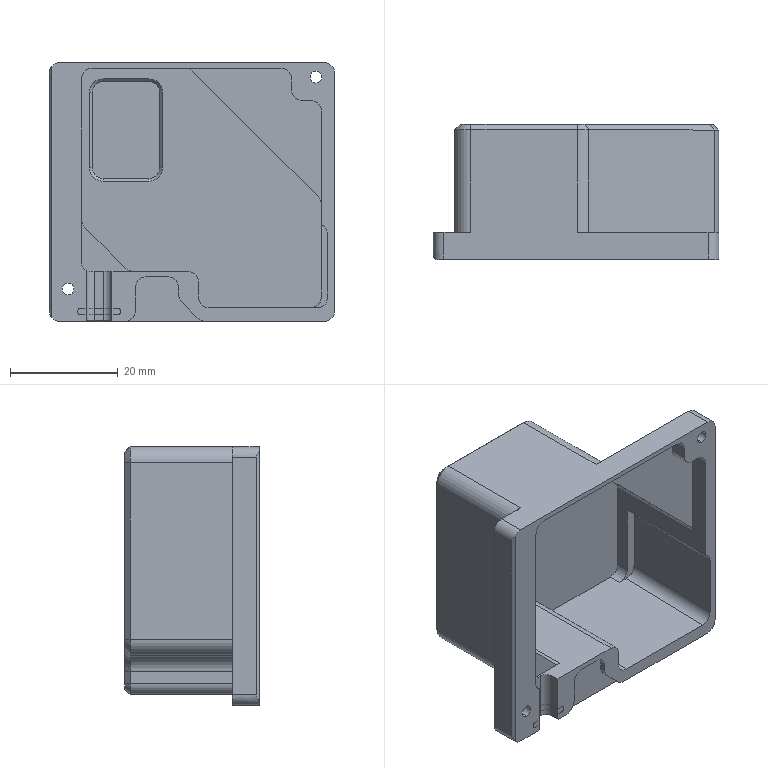NC program | NX | posted with a generic post | part box 53 x 25 x 48 mm
Lines 1 to 807 of 6007:
N10 G17 G21 G94 G90
(动态粗_COPY_1 , TOOL : D10-30-D10-75-3T-ROUGH)
N12 T02 M6
N14 G54
N16 G17 G0 G90 X35.554 Y-25.846 B0. C0. S6500 M3
N18 G43 Z30. H2
N20 Z0.65 B-180. C-180.
N22 G94 G1 X35.529 Y-25.845 Z0.494 F2000.
N24 X35.504 Z0.432
N26 X35.479 Z0.387
N28 X35.454 Z0.35
N30 X35.429 Y-25.844 Z0.319
N32 X35.404 Z0.293
N34 X35.379 Z0.27
N36 X35.354 Y-25.843 Z0.25
N38 X35.329 Z0.232
N40 X35.304 Z0.217
N42 X35.279 Y-25.842 Z0.203
N44 X35.254 Z0.192
N46 X35.229 Z0.182
N48 X35.204 Z0.173
N50 X35.179 Y-25.841 Z0.166
N52 X35.154 Z0.16
N54 X35.129 Z0.156
N56 X35.104 Y-25.84 Z0.153
N58 X35.079 Z0.151
N60 X35.054 Z0.15
N62 X33.493 Y-25.821
N64 G3 X32.52 Y-26.519 R1.01
N66 G2 X29.686 Y-30.014 R6.251
N68 X25.054 Y-31.527 R11.946
N70 X18.588 Y-31.875 R52.629
N72 G1 X10.353 Y-31.9
N74 X-25.28 Y-31.897
N76 G2 X-29.327 Y-29.833 R5.556
N78 X-31.292 Y-25.589 R9.602
N80 X-31.835 Y-19.999 R30.499
N82 X-31.9 Y-8.929 R569.83
N84 G1 Y25.234
N86 G2 X-29.888 Y29.26 R5.529
N88 X-25.557 Y31.289 R9.62
N90 X-19.876 Y31.835 R31.
N92 X-9.527 Y31.898 R571.009
N94 G1 X25.236
N96 G2 X29.291 Y29.852 R5.54
N98 X31.282 Y25.592 R9.623
N100 X31.837 Y19.867 R30.807
N102 X31.9 Y8.933 R592.
N104 G1 X31.897 Y-23.257
N106 G2 X28.977 Y-28.655 R7.012
N108 X24.113 Y-30.682 R11.786
N110 X17.89 Y-31.234 R37.55
N112 X6.28 Y-31.299 R638.037
N114 G1 X-22.94 Y-31.297
N116 G2 X-28.771 Y-28.132 R7.24
N118 X-30.725 Y-23.187 R12.228
N120 X-31.237 Y-17.095 R39.453
N122 X-31.3 Y-5.485 R667.483
N124 G1 X-31.299 Y22.914
N126 G2 X-28.051 Y28.817 R7.277
N128 X-23.128 Y30.729 R12.37
N130 X-17.036 Y31.235 R39.893
N132 X-5.426 Y31.298 R679.419
N134 G1 X22.916 Y31.297
N136 G2 X28.765 Y28.125 R7.261
N138 X30.695 Y23.312 R12.133
N140 X31.235 Y17.087 R38.508
N142 X31.299 Y5.522 R649.21
N144 G1 X31.296 Y-21.142
N146 G2 X27.232 Y-28.31 R8.281
N148 X21.996 Y-30.146 R14.249
N150 X15.045 Y-30.648 R48.883
N152 X4.02 Y-30.699 R723.913
N154 G1 X-20.915 Y-30.697
N156 G2 X-28.38 Y-26.453 R8.43
N158 X-30.181 Y-21.105 R14.722
N160 X-30.656 Y-13.971 R52.882
N162 X-30.7 Y-3.036 R735.61
N164 G1 X-30.698 Y20.889
N166 G2 X-26.451 Y28.373 R8.443
N168 X-21.059 Y30.182 R14.801
N170 X-14.285 Y30.648 R51.298
N172 X-3.261 Y30.698 R725.317
N174 G1 X20.891 Y30.696
N176 G2 X28.394 Y26.416 R8.45
N178 X30.169 Y21.152 R14.725
N180 X30.648 Y14.334 R50.321
N182 X30.699 Y3.309 R722.797
N184 G1 X30.697 Y-19.162
N186 G2 X29.691 Y-23.912 R10.114
N188 X24.852 Y-28.306 R9.826
N190 X19.019 Y-29.739 R19.275
N192 X10.84 Y-30.078 R86.406
N194 G1 X1.93 Y-30.098
N196 X-18.98 Y-30.097
N198 G2 X-23.582 Y-29.222 R10.577
N200 X-28.208 Y-24.411 R9.734
N202 X-29.701 Y-18.688 R18.552
N204 X-30.074 Y-10.69 R77.607
N206 G1 X-30.099 Y-1.285
N208 X-30.098 Y18.999
N210 G2 X-29.171 Y23.68 R10.488
N212 X-24.416 Y28.199 R9.747
N214 X-18.739 Y29.69 R18.485
N216 X-10.697 Y30.072 R76.519
N218 G1 X-1.292 Y30.097
N220 X19.001 Y30.096
N222 G2 X23.641 Y29.189 R10.513
N224 X28.183 Y24.451 R9.727
N226 X29.682 Y18.818 R18.319
N228 X30.073 Y10.641 R76.165
N230 G1 X30.098 Y1.236
N232 X30.096 Y-17.587
N234 G2 X29.384 Y-22.094 R12.32
N236 X24.486 Y-27.327 R9.973
N238 X18.589 Y-29.02 R18.202
N240 X10.596 Y-29.462 R69.268
N242 G1 X0.696 Y-29.498
N244 X-17.405 Y-29.496
N246 G2 X-21.836 Y-28.858 R12.948
N248 X-27.27 Y-23.951 R9.961
N250 X-29.001 Y-18.063 R17.971
N252 X-29.459 Y-10.205 R66.372
N254 X-29.499 Y0.729 R746.861
N256 G1 X-29.498 Y17.334
N258 G2 X-28.88 Y21.769 R13.162
N260 X-23.899 Y27.29 R9.97
N262 X-17.956 Y29.012 R18.194
N264 X-10.279 Y29.455 R66.668
N266 X0.161 Y29.497 R724.044
N268 G1 X17.381 Y29.495
N270 G2 X21.77 Y28.878 R13.073
N272 X27.22 Y24.034 R9.935
N274 X28.985 Y18.159 R17.739
N276 X29.458 Y10.168 R65.522
N278 X29.498 Y-0.722 R745.473
N280 G1 X29.496 Y-15.832
N282 G2 X29.047 Y-20.16 R16.314
N284 X23.818 Y-26.522 R10.259
N286 X17.949 Y-28.329 R18.072
N288 X10.006 Y-28.847 R62.201
N290 X-0.884 Y-28.897 R721.33
N292 G1 X-15.785 Y-28.896
N294 G2 X-20.243 Y-28.409 R16.17
N296 X-26.532 Y-23.161 R10.318
N298 X-28.337 Y-17.249 R18.219
N300 X-28.846 Y-9.441 R62.288
N302 X-28.898 Y1.494 R719.311
N304 G1 X-28.897 Y15.894
N306 G2 X-28.364 Y20.391 R15.5
N308 X-23.157 Y26.528 R10.343
N310 X-17.281 Y28.328 R18.221
N312 X-9.518 Y28.842 R61.43
N314 X2.406 Y28.897 R750.329
N316 G1 X15.716 Y28.896
N318 G2 X20.177 Y28.425 R16.524
N320 X26.482 Y23.244 R10.301
N322 X28.326 Y17.298 R18.066
N324 X28.843 Y9.536 R61.154
N326 X28.897 Y-2.389 R749.38
N328 G1 X28.896 Y-14.392
N330 G2 X28.477 Y-18.951 R19.03
N332 X23.029 Y-25.813 R10.642
N334 X16.862 Y-27.715 R18.687
N336 X8.74 Y-28.244 R64.249
N338 X-3.14 Y-28.297 R757.56
N340 X-15.694 Y-28.273 R887.318
N342 X-20.816 Y-27.214 R12.969
N344 X-26.074 Y-21.885 R11.022
N346 X-27.805 Y-15.573 R20.29
N348 X-28.259 Y-7.219 R75.925
N350 X-28.298 Y4.165 R769.566
N352 X-28.272 Y15.759 R817.448
N354 X-27.127 Y20.994 R12.746
N356 X-21.786 Y26.117 R11.092
N358 X-15.777 Y27.775 R20.162
N360 X-7.786 Y28.248 R70.147
N362 X3.149 Y28.296 R730.798
N364 X15.671 Y28.273 R887.366
N366 X20.754 Y27.238 R13.038
N368 X26.082 Y21.86 R11.015
N370 X27.8 Y15.589 R20.309
N372 X28.257 Y7.236 R75.377
N374 X28.297 Y-4.149 R767.6
N376 X28.261 Y-14.841 R508.587
N378 X27.086 Y-20.164 R13.26
N380 X21.611 Y-25.448 R11.373
N382 X15.257 Y-27.183 R20.829
N384 X6.904 Y-27.652 R75.577
N386 X-4.48 Y-27.697 R761.549
N388 X-14.704 Y-27.664 R547.958
N390 X-19.955 Y-26.568 R13.604
N392 X-25.43 Y-21.018 R11.365
N394 X-27.171 Y-14.711 R20.759
N396 X-27.651 Y-6.405 R73.707
N398 X-27.698 Y5.475 R773.48
N400 X-27.656 Y14.903 R355.222
N402 X-26.381 Y20.339 R13.066
N404 X-20.836 Y25.511 R11.506
N406 X-14.555 Y27.188 R21.209
N408 X-5.932 Y27.656 R78.328
N410 X5.453 Y27.696 R772.917
N412 X14.816 Y27.658 R400.806
N414 X20.179 Y26.459 R13.284
N416 X25.494 Y20.875 R11.462
N418 X27.195 Y14.503 R21.268
N420 X27.657 Y5.925 R78.807
N422 X27.697 Y-5.46 R768.724
N424 X27.653 Y-13.851 R267.429
N426 X26.512 Y-19.185 R13.994
N428 X20.92 Y-24.736 R11.617
N430 X14.492 Y-26.542 R20.953
N432 X6.007 Y-27.046 R73.691
N434 X-13.309 Y-27.071 R950.623
N436 X-18.519 Y-26.179 R15.541
N438 X-24.632 Y-20.498 R11.491
N440 X-26.477 Y-14.312 R20.187
N442 X-27.034 Y-6.057 R65.857
N444 X-27.067 Y13.464 R849.746
N446 X-26.087 Y18.744 R14.979
N448 X-20.394 Y24.681 R11.558
N450 X-14.107 Y26.503 R20.57
N452 X-5.534 Y27.042 R70.432
N454 X13.466 Y27.065 R870.105
N456 X18.705 Y26.102 R15.02
N458 X24.616 Y20.521 R11.51
N460 X26.51 Y14.068 R20.462
N462 X27.043 Y5.54 R70.671
N464 X27.061 Y-12.546 R717.329
N466 X26.103 Y-17.833 R15.664
N468 X20.292 Y-24.005 R11.768
N470 X13.931 Y-25.876 R20.77
N472 X5.539 Y-26.433 R68.355
N474 X-12.544 Y-26.458 R650.416
N476 X-17.872 Y-25.477 R15.602
N478 X-23.962 Y-19.752 R11.777
N480 X-25.876 Y-13.301 R20.711
N482 X-26.439 Y-4.64 R69.842
N484 X-26.467 Y12.324 R743.336
N486 X-25.587 Y17.581 R16.346
N488 X-19.793 Y23.937 R11.741
N490 X-13.261 Y25.879 R20.723
N492 X-4.734 Y26.435 R69.618
N494 X12.545 Y26.458 R613.963
N496 X17.915 Y25.456 R15.556
N498 X24.029 Y19.61 R11.828
N500 X25.876 Y13.281 R20.935
N502 X26.435 Y4.755 R69.201
N504 X26.456 Y-11.579 R549.883
N506 X25.515 Y-16.917 R16.448
N508 X19.633 Y-23.302 R11.978
N510 X13.057 Y-25.26 R21.03
N512 X4.577 Y-25.829 R69.067
N514 X-11.533 Y-25.856 R521.856
N516 X-16.872 Y-24.923 R16.563
N518 X-23.291 Y-19.032 R11.993
N520 X-25.249 Y-12.502 R20.966
N522 X-25.833 Y-3.752 R69.591
N524 X-25.855 Y11.592 R472.715
N526 X-24.867 Y17.011 R16.272
N528 X-18.972 Y23.317 R12.026
N530 X-12.347 Y25.269 R21.256
N532 X-3.866 Y25.829 R70.201
N534 X11.433 Y25.859 R523.962
N536 X16.82 Y24.939 R16.819
N538 X23.334 Y18.94 R12.02
N540 X25.281 Y12.27 R21.393
N542 X25.836 Y3.563 R72.503
N544 X25.854 Y-10.566 R447.25
N546 X24.95 Y-15.957 R17.405
N548 X18.96 Y-22.617 R12.165
N550 X12.351 Y-24.624 R21.127
N552 X4.008 Y-25.218 R66.68
N554 X-10.571 Y-25.252 R411.854
N556 X-15.961 Y-24.341 R17.389
N558 X-22.653 Y-18.269 R12.214
N560 X-24.621 Y-11.741 R21.273
N562 X-25.219 Y-3.353 R66.767
N564 X-25.252 Y10.596 R382.106
N566 X-24.299 Y16.069 R17.14
N568 X-18.314 Y22.626 R12.213
N570 X-11.703 Y24.623 R21.241
N572 X-3.225 Y25.219 R67.682
N574 X10.59 Y25.251 R382.034
N576 X15.978 Y24.332 R17.299
N578 X22.638 Y18.288 R12.205
N580 X24.629 Y11.673 R21.309
N582 X25.225 Y3.014 R68.932
N584 X25.249 Y-9.675 R342.573
N586 X24.319 Y-15.199 R17.91
N588 X18.199 Y-21.987 R12.387
N590 X11.454 Y-24.02 R21.579
N592 X2.571 Y-24.626 R70.663
N594 X-9.713 Y-24.645 R315.185
N596 X-15.107 Y-23.744 R17.961
N598 X-21.977 Y-17.599 R12.4
N600 X-24.014 Y-10.867 R21.573
N602 X-24.623 Y-2.074 R69.823
N604 X-24.643 Y9.805 R280.992
N606 X-23.649 Y15.361 R17.395
N608 X-17.493 Y22.027 R12.445
N610 X-10.789 Y24.023 R21.799
N612 X-2.086 Y24.621 R70.222
N614 X9.703 Y24.645 R295.153
N616 X15.139 Y23.73 R17.899
N618 X21.984 Y17.576 R12.401
N620 X24.003 Y10.923 R21.528
N622 X24.623 Y2.041 R69.447
N624 X24.632 Y-9.073 R234.056
N626 X23.592 Y-14.711 R17.521
N628 X17.312 Y-21.429 R12.635
N630 X10.561 Y-23.419 R22.218
N632 X1.857 Y-24.019 R71.006
N634 X-8.986 Y-24.033 R230.606
N636 X-14.504 Y-23.063 R17.92
N638 X-21.394 Y-16.765 R12.623
N640 X-23.421 Y-9.923 R22.193
N642 X-24.023 Y-1.039 R72.238
N644 X-24.023 Y9.22 R192.786
N646 X-22.912 Y14.889 R17.024
N648 X-16.703 Y21.422 R12.677
N650 X-9.857 Y23.428 R22.381
N652 X-1.243 Y24.017 R71.555
N654 X9.016 Y24.031 R210.635
N656 X14.617 Y23.018 R17.689
N658 X21.402 Y16.74 R12.64
N660 X23.422 Y9.901 R22.259
N662 X24.016 Y1.332 R70.641
N664 X24.01 Y-8.521 R164.838
N666 X22.829 Y-14.312 R17.035
N668 X16.643 Y-20.768 R12.835
N670 X9.896 Y-22.786 R22.297
N672 X1.285 Y-23.409 R69.015
N674 X-8.389 Y-23.414 R166.145
N676 X-14.146 Y-22.289 R17.398
N678 X-20.734 Y-16.092 R12.81
N680 X-22.795 Y-9.221 R22.307
N682 X-23.412 Y-0.564 R69.981
N684 X-23.402 Y8.615 R140.392
N686 X-22.165 Y14.437 R16.715
N688 X-15.99 Y20.783 R12.874
N690 X-9.279 Y22.783 R22.396
N692 X-0.398 Y23.414 R70.327
N694 X8.511 Y23.406 R144.104
N696 X14.259 Y22.24 R17.066
N698 X20.811 Y15.933 R12.871
N700 X22.818 Y9.048 R22.752
N702 X23.418 Y0.254 R72.774
N704 X23.379 Y-8.069 R112.025
N706 X22.038 Y-13.959 R16.459
N708 X15.754 Y-20.224 R13.084
N710 X8.907 Y-22.206 R23.071
N712 X-0.111 Y-22.818 R73.983
N714 X-8.209 Y-22.766 R101.749
N716 X-14.21 Y-21.311 R16.044
N718 X-20.296 Y-14.989 R13.189
N720 X-22.229 Y-8.127 R23.515
N722 X-22.826 Y1.073 R77.274
N724 X-22.736 Y8.584 R80.685
N726 X-21.034 Y14.742 R15.233
N728 X-14.758 Y20.401 R13.357
N730 X-7.876 Y22.261 R24.222
N732 X1.552 Y22.833 R82.25
N734 X8.703 Y22.724 R74.231
N736 X14.923 Y20.932 R14.989
N738 X20.436 Y14.681 R13.421
N740 X22.275 Y7.783 R24.476
N742 X22.833 Y-1.555 R82.512
N744 X22.685 Y-8.255 R60.76
N746 X20.62 Y-14.712 R14.668
N748 X14.36 Y-19.913 R13.755
N750 X7.364 Y-21.702 R25.44
N752 X-2.291 Y-22.238 R88.472
N754 X-8.762 Y-22.023 R49.25
N756 X-15.504 Y-19.466 R13.946
N758 X-20.119 Y-13.256 R14.226
N760 X-21.766 Y-6.223 R27.118
N762 X-22.155 Y7.349 R94.133
N764 X-20.786 Y13.278 R16.544
N766 X-14.474 Y19.569 R13.237
N768 X-7.497 Y21.595 R23.333
N770 X1.881 Y22.219 R75.892
N772 X8.579 Y22.042 R52.749
N774 X15.249 Y19.647 R14.131
N776 X20.039 Y13.441 R14.06
N778 X21.761 Y6.242 R26.799
N780 X22.149 Y-6.52 R87.365
N782 X20.801 Y-12.503 R16.905
N784 X14.432 Y-18.923 R13.335
N786 X7.408 Y-20.98 R23.416
N788 X-2.059 Y-21.614 R74.623
N790 X-8.437 Y-21.347 R40.943
N792 X-15.787 Y-18.035 R13.586
N794 X-19.806 Y-11.722 R15.207
N796 X-21.275 Y-4.322 R31.024
N798 X-21.531 Y6.646 R79.918
N800 X-20.06 Y12.781 R16.428
N802 X-13.65 Y19.002 R13.43
N804 X-6.706 Y20.989 R23.815
N806 X3.437 Y21.614 R76.356
N808 X9.396 Y21.177 R29.883
N810 X18.824 Y14.007 R13.224
N812 X20.944 Y7.01 R22.917
N814 X21.504 Y-6.098 R69.517
N816 X19.897 Y-12.378 R16.169
N818 X13.476 Y-18.425 R13.622
N820 X6.299 Y-20.422 R24.494
N822 X-6.095 Y-20.899 R69.072
N824 X-12.374 Y-19.29 R16.152
N826 X-18.426 Y-12.86 R13.633
N828 X-20.389 Y-5.914 R24.213
N830 X-20.884 Y6.208 R64.057
N832 X-19.234 Y12.477 R15.904
N834 X-12.923 Y18.392 R13.619
N836 X-6.022 Y20.37 R24.002
N838 X6.279 Y20.877 R63.529
N840 X12.576 Y19.18 R15.764
N842 X18.462 Y12.776 R13.691
N844 X20.4 Y5.823 R24.456
N846 X20.87 Y-5.445 R59.567
N848 X19.208 Y-11.803 R16.066
N850 X12.854 Y-17.767 R13.723
N852 X5.777 Y-19.781 R24.301
N854 X-5.535 Y-20.257 R58.096
N856 X-11.958 Y-18.517 R15.853
N858 X-17.822 Y-12.127 R13.798
N860 X-19.812 Y-4.952 R24.79
N862 X-20.231 Y5.732 R53.722
N864 X-18.416 Y12.134 R15.496
N866 X-12.143 Y17.81 R13.817
N868 X-5.103 Y19.787 R24.537
N870 X5.67 Y20.235 R53.981
N872 X12.08 Y18.446 R15.592
N874 X17.851 Y12.056 R13.838
N876 X19.802 Y5.005 R24.809
N878 X20.211 Y-5.005 R49.739
N880 X18.331 Y-11.57 R15.535
N882 X11.936 Y-17.254 R13.978
N884 X4.795 Y-19.208 R25.17
N886 X-5.081 Y-19.598 R48.664
N888 X-11.635 Y-17.685 R15.423
N890 X-17.25 Y-11.333 R13.997
N892 X-19.213 Y-4.146 R25.202
N894 X-19.571 Y5.235 R45.062
N896 X-17.546 Y11.858 R15.1
N898 X-11.181 Y17.315 R14.091
N900 X-3.942 Y19.238 R25.717
N902 X5.262 Y19.567 R44.819
N904 X11.947 Y17.492 R15.038
N906 X17.303 Y11.207 R14.104
N908 X19.246 Y3.878 R25.719
N910 X19.517 Y-4.831 R40.357
N912 X17.191 Y-11.709 R14.716
N914 X10.838 Y-16.819 R14.415
N916 X3.488 Y-18.675 R26.738
N918 X-4.818 Y-18.91 R39.579
N920 X-11.704 Y-16.586 R14.705
N922 X-16.817 Y-10.23 R14.429
N924 X-18.679 Y-2.832 R26.756
N926 X-18.857 Y5.159 R35.852
N928 X-16.086 Y12.388 R14.197
N930 X-9.759 Y17.01 R14.867
N932 X-2.282 Y18.74 R28.316
N934 X5.351 Y18.833 R34.445
N936 X12.85 Y15.711 R13.965
N938 X17.194 Y9.285 R15.293
N940 X18.819 Y1.418 R29.998
N942 X18.693 Y-5.449 R28.369
N944 X11.386 Y-15.608 R13.603
N946 X4.144 Y-17.869 R23.229
N948 X-4.51 Y-18.212 R33.936
N950 X-11.854 Y-15.354 R14.16
N952 X-16.414 Y-9.027 R14.997
N954 X-18.172 Y-1.057 R28.528
N956 X-18.019 Y5.717 R26.107
N958 X-10.798 Y15.59 R13.545
N960 X-3.793 Y17.821 R22.844
N962 X4.59 Y18.179 R31.874
N964 X12.237 Y15.03 R13.931
N966 X16.573 Y8.608 R15.372
N968 X18.241 Y-0.341 R29.575
N970 X17.56 Y-6.844 R19.731
N972 X10.853 Y-14.909 R13.532
N974 X3.636 Y-17.22 R22.702
N976 X-4.209 Y-17.497 R28.634
N978 X-12.539 Y-13.5 R13.652
N980 X-16.317 Y-6.888 R16.547
N982 X-17.482 Y4.095 R28.29
N984 X-13.609 Y12.422 R13.611
N986 X-6.994 Y16.278 R16.381
N988 X3.984 Y17.492 R28.404
N990 X12.014 Y13.999 R13.703
N992 X16.087 Y7.559 R15.795
N994 X17.423 Y-3.529 R26.408
N996 X10.096 Y-14.332 R13.584
N998 X2.384 Y-16.676 R22.888
N1000 X-4.873 Y-16.603 R22.372
N1002 X-14.176 Y-9.769 R13.457
N1004 X-16.626 Y-2.046 R22.077
N1006 X-16.522 Y5.117 R20.972
N1008 X-9.831 Y14.134 R13.375
N1010 X-2.205 Y16.6 R21.877
N1012 X5.049 Y16.534 R21.209
N1014 X14.186 Y9.738 R13.392
N1016 X16.647 Y1.689 R21.811
N1018 X16.266 Y-5.323 R18.599
N1020 X9.715 Y-13.549 R13.388
N1022 X1.589 Y-16.038 R21.801
N1024 X-5.464 Y-15.616 R18.308
N1026 X-13.563 Y-9.079 R13.393
N1028 X-16.104 Y0.228 R21.621
N1030 X-14.902 Y7.349 R15.386
N1032 X-8.605 Y13.81 R13.626
N1034 X3.499 Y15.977 R21.569
N1036 X13.494 Y9.182 R13.285
N1038 X15.881 Y-3.077 R20.281
N1040 X9.248 Y-12.806 R13.214
N1042 X-2.993 Y-15.279 R20.212
N1044 X-12.802 Y-8.641 R13.195
N1046 X-15.206 Y3.113 R19.25
N1048 X-8.715 Y12.747 R13.073
N1050 X3.213 Y15.189 R19.179
N1052 X12.77 Y8.671 R13.07
N1054 X15.101 Y-2.643 R18.197
N1056 X8.771 Y-12.059 R12.968
N1058 X-2.604 Y-14.49 R18.113
N1060 X-12.076 Y-8.127 R12.948
N1062 X-14.396 Y2.772 R17.235
N1064 X-8.201 Y12.017 R12.803
N1066 X2.775 Y14.392 R17.202
N1068 X12.04 Y8.152 R12.785
N1070 X14.282 Y-2.262 R16.313
N1072 X8.219 Y-11.346 R12.662
N1074 X-2.314 Y-13.657 R16.208
N1076 X-11.357 Y-7.579 R12.627
N1078 X-13.547 Y2.484 R15.417
N1080 X-7.736 Y11.24 R12.446
N1082 X2.557 Y13.531 R15.362
N1084 X11.349 Y7.545 R12.439
N1086 X13.382 Y-2.181 R14.537
N1088 X7.608 Y-10.652 R12.298
N1090 X-2.172 Y-12.765 R14.45
N1092 X-10.701 Y-6.9 R12.244
N1094 X-12.613 Y2.476 R13.715
N1096 X-6.985 Y10.622 R12.065
N1098 X2.414 Y12.617 R13.673
N1100 X10.814 Y6.634 R12.028
N1102 X12.359 Y-2.479 R12.842
N1104 X6.468 Y-10.25 R11.95
N1106 X-2.651 Y-11.699 R12.692
N1108 X-10.422 Y-5.488 R11.878
N1110 X-11.291 Y3.717 R11.899
N1112 X-4.784 Y10.737 R11.89
N1114 X4.742 Y10.886 R11.618
N1116 X11.523 Y-1.516 R11.805
N1118 X5.466 Y-9.7 R11.274
N1120 X-4.723 Y-9.854 R11.075
N1122 X-10.766 Y1.34 R11.236
N1124 X-4.466 Y9.799 R10.863
N1126 X9.663 Y4.585 R10.526
N1128 X5.723 Y-8.372 R10.193
N1130 X-9.716 Y0.793 R10.031
N1132 X1.784 Y9.554 R9.798
N1134 X9.424 Y-0.479 R9.411
N1136 X-1.26 Y-8.664 R9.175
N1138 X-8.514 Y0.552 R8.78
N1140 X1.68 Y8.303 R8.52
N1142 X7.891 Y-1.627 R8.064
N1144 X-3.519 Y-6.394 R7.748
N1146 X-3.407 Y6.137 R7.21
N1148 X5.869 Y3.276 R6.707
N1150 X2.267 Y-5.373 R6.199
N1152 X-4.674 Y-1.997 R5.514
N1154 X-2.974 Y3.444 R4.718
N1156 X-0.363 Y4.153 R4.737
N1158 G1 X-0.338 Y4.154 Z0.151
N1160 X-0.313 Y4.155 Z0.153
N1162 X-0.288 Y4.157 Z0.156
N1164 X-0.263 Y4.158 Z0.16
N1166 X-0.238 Y4.159 Z0.166
N1168 X-0.213 Y4.16 Z0.173
N1170 X-0.188 Y4.161 Z0.182
N1172 X-0.163 Y4.162 Z0.192
N1174 X-0.138 Y4.164 Z0.203
N1176 X-0.113 Y4.165 Z0.217
N1178 X-0.088 Y4.166 Z0.232
N1180 X-0.063 Y4.167 Z0.25
N1182 X-0.038 Y4.168 Z0.27
N1184 X-0.013 Y4.169 Z0.293
N1186 X0.012 Y4.171 Z0.319
N1188 X0.037 Y4.172 Z0.35
N1190 X0.062 Y4.173 Z0.387
N1192 X0.087 Y4.174 Z0.432
N1194 X0.112 Y4.175 Z0.494
N1196 X0.137 Y4.176 Z0.65
N1198 G0 Z30.
(动态粗_COPY_1_COPY , TOOL : D10-30-D10-75-3T-ROUGH)
N1200 X-0.119 Y0.416
N1202 Z0.5
N1204 G3 X-0.119 Y0.416 Z0.006 I-2.039 J-4.011
N1206 X-0.119 Y0.416 Z-0.487 I-2.039 J-4.011
N1208 X-0.119 Y0.416 Z-0.981 I-2.039 J-4.011
N1210 X-0.119 Y0.416 Z-1.474 I-2.039 J-4.011
N1212 X-0.119 Y0.416 Z-1.968 I-2.039 J-4.011
N1214 X-0.119 Y0.416 Z-2.461 I-2.039 J-4.011
N1216 X-0.119 Y0.416 Z-2.955 I-2.039 J-4.011
N1218 X-0.119 Y0.416 Z-3.448 I-2.039 J-4.011
N1220 X-0.119 Y0.416 Z-3.942 I-2.039 J-4.011
N1222 X-0.119 Y0.416 Z-4.435 I-2.039 J-4.011
N1224 X-0.119 Y0.416 Z-4.929 I-2.039 J-4.011
N1226 X-0.119 Y0.416 Z-5.422 I-2.039 J-4.011
N1228 X-0.119 Y0.416 Z-5.916 I-2.039 J-4.011
N1230 X-0.119 Y0.416 Z-6.409 I-2.039 J-4.011
N1232 X-0.119 Y0.416 Z-6.903 I-2.039 J-4.011
N1234 X-0.119 Y0.416 Z-7.396 I-2.039 J-4.011
N1236 X-0.119 Y0.416 Z-7.89 I-2.039 J-4.011
N1238 X-0.119 Y0.416 Z-8.384 I-2.039 J-4.011
N1240 X-0.119 Y0.416 Z-8.877 I-2.039 J-4.011
N1242 X-0.119 Y0.416 Z-9.371 I-2.039 J-4.011
N1244 X-0.119 Y0.416 Z-9.864 I-2.039 J-4.011
N1246 X-0.119 Y0.416 Z-10.358 I-2.039 J-4.011
N1248 X-0.119 Y0.416 Z-10.851 I-2.039 J-4.011
N1250 X-0.119 Y0.416 Z-11.345 I-2.039 J-4.011
N1252 X-0.119 Y0.416 Z-11.838 I-2.039 J-4.011
N1254 X-0.119 Y0.416 Z-12.332 I-2.039 J-4.011
N1256 X-0.119 Y0.416 Z-12.825 I-2.039 J-4.011
N1258 X-0.119 Y0.416 Z-13.319 I-2.039 J-4.011
N1260 X-0.119 Y0.416 Z-13.812 I-2.039 J-4.011
N1262 X-0.119 Y0.416 Z-14.306 I-2.039 J-4.011
N1264 X-0.119 Y0.416 Z-14.799 I-2.039 J-4.011
N1266 X-0.119 Y0.416 Z-15.293 I-2.039 J-4.011
N1268 X-0.119 Y0.416 Z-15.787 I-2.039 J-4.011
N1270 X-0.119 Y0.416 Z-16.28 I-2.039 J-4.011
N1272 X-0.119 Y0.416 Z-16.774 I-2.039 J-4.011
N1274 X-0.119 Y0.416 Z-17.267 I-2.039 J-4.011
N1276 X-0.119 Y0.416 Z-17.761 I-2.039 J-4.011
N1278 X-0.119 Y0.416 Z-18.254 I-2.039 J-4.011
N1280 X-0.119 Y0.416 Z-18.748 I-2.039 J-4.011
N1282 X-0.119 Y0.416 Z-19.241 I-2.039 J-4.011
N1284 X-0.119 Y0.416 Z-19.735 I-2.039 J-4.011
N1286 X-0.119 Y0.416 Z-20.228 I-2.039 J-4.011
N1288 X-0.119 Y0.416 Z-20.722 I-2.039 J-4.011
N1290 X-0.119 Y0.416 Z-21.215 I-2.039 J-4.011
N1292 X-0.119 Y0.416 Z-21.709 I-2.039 J-4.011
N1294 X-0.119 Y0.416 Z-22.202 I-2.039 J-4.011
N1296 X-0.119 Y0.416 Z-22.696 I-2.039 J-4.011
N1298 X-6.658 Y-3.596 Z-22.856 R4.5
N1300 X-0.229 Y0.526 R-4.525
N1302 X-6.526 Y-2.169 R4.623
N1304 X-1.303 Y-8.313 R4.631
N1306 X-6.185 Y-0.9 R-4.819
N1308 X-0.466 Y-8.381 R4.934
N1310 X-6.13 Y-0.347 R-5.102
N1312 X0.231 Y-8.4 R5.234
N1314 X-6.265 Y-0.053 R-5.393
N1316 X0.564 Y-8.561 R5.532
N1318 X-6.283 Y0.37 R-5.691
N1320 X0.762 Y-8.803 R5.837
N1322 X-6.158 Y0.915 R-5.998
N1324 X0.811 Y-9.131 R6.149
N1326 X-6.077 Y1.391 R-6.311
N1328 X1.196 Y-9.282 R6.469
N1330 X-6.286 Y1.64 R-6.634
N1332 X1.188 Y-9.664 R6.794
N1334 X-6.12 Y2.169 R-6.962
N1336 X1.274 Y-9.998 R7.127
N1338 X-6.025 Y2.633 R-7.297
N1340 X0.644 Y-10.665 R7.465
N1342 X-5.752 Y3.183 R-7.638
N1344 X0.362 Y-11.137 R7.81
N1346 X-5.564 Y3.666 R-7.985
N1348 X0.185 Y-11.562 R8.161
N1350 X-5.482 Y4.094 R-8.34
N1352 X-0.182 Y-12.028 R8.517
N1354 X-4.915 Y4.694 R-8.698
N1356 X-0.426 Y-12.452 R8.879
N1358 X-4.128 Y5.29 R-9.062
N1360 X-1.193 Y-12.935 R9.245
N1362 X-2.103 Y5.869 R9.427
N1364 X-1.49 Y-13.335 R-9.614
N1366 X-0.844 Y6.158 R9.802
N1368 X-2.67 Y-13.721 R-9.989
N1370 X1.923 Y5.771 R10.176
N1372 X-7.054 Y-12.88 R10.358
N1374 X5.399 Y3.826 R10.541
N1376 X-12.844 Y-2.349 R10.702
N1378 X7.079 Y-9.485 R10.845
N1380 X-9.027 Y5.076 R11.013
N1382 X0.939 Y-14.495 R11.19
N1384 X-4.303 Y7.63 R11.38
N1386 X-5.01 Y-14.946 R11.567
N1388 X9.55 Y-4.909 R11.723
N1390 X9.486 Y-1.983 R26.733
N1392 X-9.136 Y6.01 R11.798
N1394 X-11.618 Y3.498 R73.491
N1396 X-13.928 Y-6.008 R11.479
N1398 X-5.294 Y-15.295 R11.997
N1400 X0.454 Y-15.282 R231.195
N1402 X5.429 Y-13.12 R9.931
N1404 X9.541 Y-7.023 R11.991
N1406 G1 X9.55 Y-4.909
N1408 X9.538 Y-7.226
N1410 G2 X8.165 Y-10.523 R8.205
N1412 X1.707 Y-15.28 R11.402
N1414 X0.166 Y-15.3 R21.461
N1416 G3 X2.26 Y-15.276 R27.12
N1418 X4.926 Y-14.22 R6.852
N1420 X8.243 Y-10.88 R509.253
N1422 X9.534 Y-8.603 R6.781
N1424 G1 X9.55 Y-7.029
N1426 G2 X9.529 Y-8.763 R17.563
N1428 X8.902 Y-10.244 R3.992
N1430 G1 X8.074 Y-11.071
N1432 G3 X9.277 Y-9.832 R16.97
N1434 X9.55 Y-9.079 R1.264
N1436 G1 Y-8.584
N1438 G2 X9.455 Y-9.557 R2.587
N1440 X9.122 Y-10.023 R1.985
N1442 G1 X4.678 Y-14.451
N1444 G2 X2.881 Y-15.3 R4.015
N1446 G1 X1.981
N1448 G3 X3.453 Y-15.265 R9.147
N1450 X4.212 Y-14.934 R1.523
N1452 G1 X4.816 Y-14.33
N1454 G2 X3.986 Y-15.109 R6.519
N1456 X3.151 Y-15.3 R1.436
N1458 G1 X-5.545 Y-15.288
N1460 G2 X-9.023 Y-13.846 R8.391
N1462 X-12.69 Y2.421 R12.112
N1464 X-11.372 Y3.774 R19.871
N1466 G3 X-13.128 Y1.989 R58.931
N1468 X-14.677 Y-1.961 R8.618
N1470 X-7.844 Y-14.989 R12.427
N1472 X-6.939 Y-15.3 R2.973
N1474 G1 X-5.364
N1476 G2 X-7.231 Y-15.281 R34.203
N1478 X-10.092 Y-13.882 R7.184
N1480 X-14.612 Y-0.536 R12.579
N1482 X-13.771 Y1.374 R6.47
N1484 G1 X-12.944 Y2.202
N1486 G3 X-14.256 Y0.829 R14.031
N1488 X-15.42 Y-2.761 R7.826
N1490 X-9.679 Y-14.668 R12.793
N1492 X-8.33 Y-15.294 R4.332
N1494 G1 X-7.049 Y-15.3
N1496 G2 X-8.554 Y-15.277 R12.224
N1498 X-11.058 Y-13.937 R6.358
N1500 X-15.54 Y-1.889 R12.863
N1502 X-14.705 Y0.436 R6.48
N1504 G1 X-14.007 Y1.138
N1506 G3 X-15.126 Y-0.05 R9.685
N1508 X-16.099 Y-3.363 R7.153
N1510 X-11.138 Y-14.398 R13.001
N1512 X-9.569 Y-15.278 R5.56
N1514 X-8.322 Y-15.3 R12.808
N1516 G2 X-9.691 Y-15.276 R9.919
N1518 X-12.001 Y-13.965 R5.802
N1520 X-16.291 Y-2.861 R12.964
N1522 X-15.527 Y-0.395 R6.598
N1524 G1 X-14.898 Y0.248
N1526 G3 X-15.886 Y-0.814 R7.927
N1528 X-16.751 Y-4.014 R6.698
N1530 X-12.221 Y-14.315 R12.987
N1532 X-10.594 Y-15.281 R4.915
N1534 X-9.464 Y-15.3 R26.284
N1536 G2 X-10.742 Y-15.272 R9.05
N1538 X-12.976 Y-13.925 R5.542
N1540 X-16.969 Y-3.68 R12.908
N1542 X-16.267 Y-1.142 R6.48
N1544 G1 X-15.641 Y-0.495
N1546 G3 X-16.585 Y-1.511 R6.836
N1548 X-17.375 Y-4.551 R6.285
N1550 X-13.215 Y-14.257 R12.796
N1552 X-11.593 Y-15.276 R4.909
N1554 X-10.515 Y-15.3 R8.814
N1556 G2 X-11.706 Y-15.273 R7.118
N1558 X-13.9 Y-13.897 R5.278
N1560 X-17.593 Y-4.226 R12.637
N1562 X-16.942 Y-1.817 R5.986
N1564 G1 X-16.35 Y-1.204
N1566 G3 X-17.272 Y-2.213 R6.192
N1568 X-17.8 Y-3.674 R4.394
N1570 X-17.774 Y-6.967 R58.064
N1572 X-13.863 Y-14.462 R11.746
N1574 X-12.5 Y-15.28 R3.943
N1576 X-11.495 Y-15.3 R17.914
N1578 G2 X-12.644 Y-15.27 R7.05
N1580 X-14.763 Y-13.895 R5.085
N1582 X-17.8 Y-8.23 R11.571
N1584 G1 Y-6.565
N1586 G3 X-17.765 Y-9.142 R28.03
N1588 X-14.105 Y-14.922 R9.126
N1590 X-13.229 Y-15.3 R1.904
N1592 G1 X-12.419
N1594 G2 X-13.516 Y-15.272 R6.141
N1596 X-15.545 Y-13.931 R4.77
N1598 X-17.793 Y-9.999 R8.972
N1600 G1 X-17.8 Y-8.75
N1602 G3 X-17.774 Y-10.566 R18.703
N1604 X-14.513 Y-15.169 R6.937
N1606 X-14.053 Y-15.3 R1.537